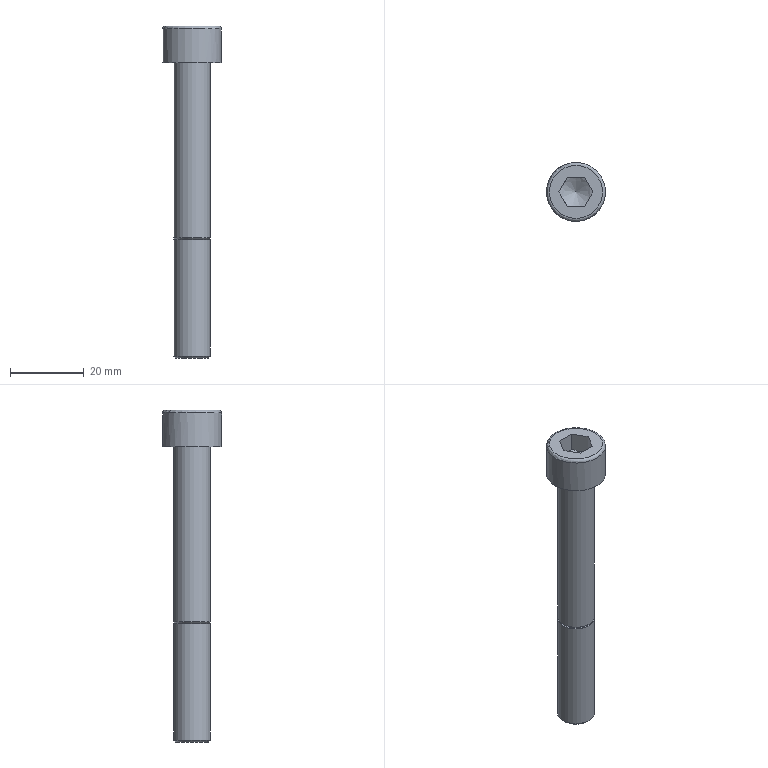Part | STEP file | 1_31 | 1 solid | 17 faces | box 16 x 16 x 90 mm | volume 7943 mm3 | plane 10 | cylinder 3 | cone 3 | torus 1 | commonest cylinder face diameters 10 x2 16 x1